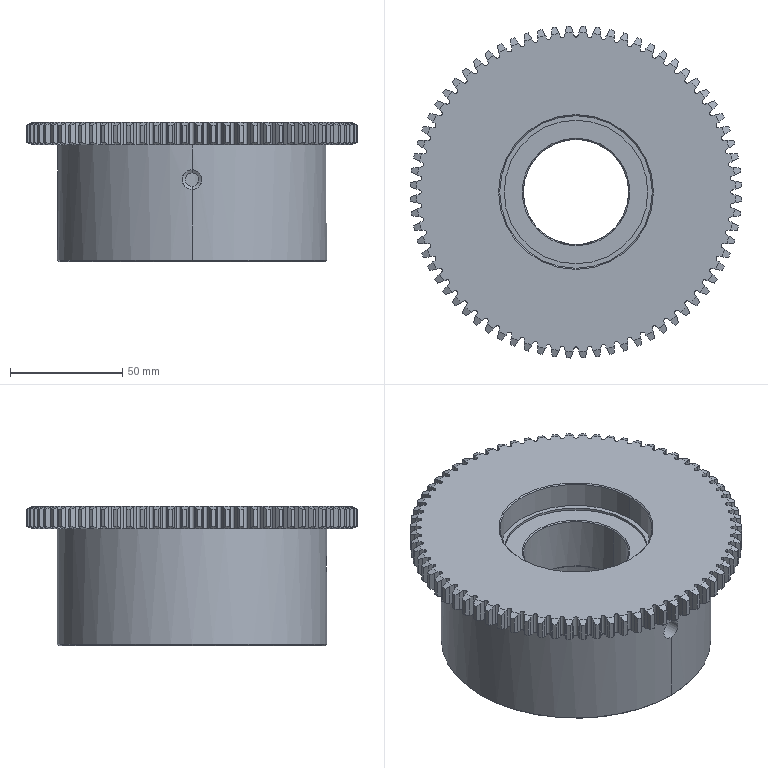Part | STEP file | 06-21 Rotor | 1 solid | 656 faces | box 147.929 x 147.929 x 62 mm | volume 569803 mm3 | plane 295 | cylinder 197 | cone 164 | commonest cylinder face diameters 2 x101 148 x72 3.3 x8 64 x4 68 x4 6 x2